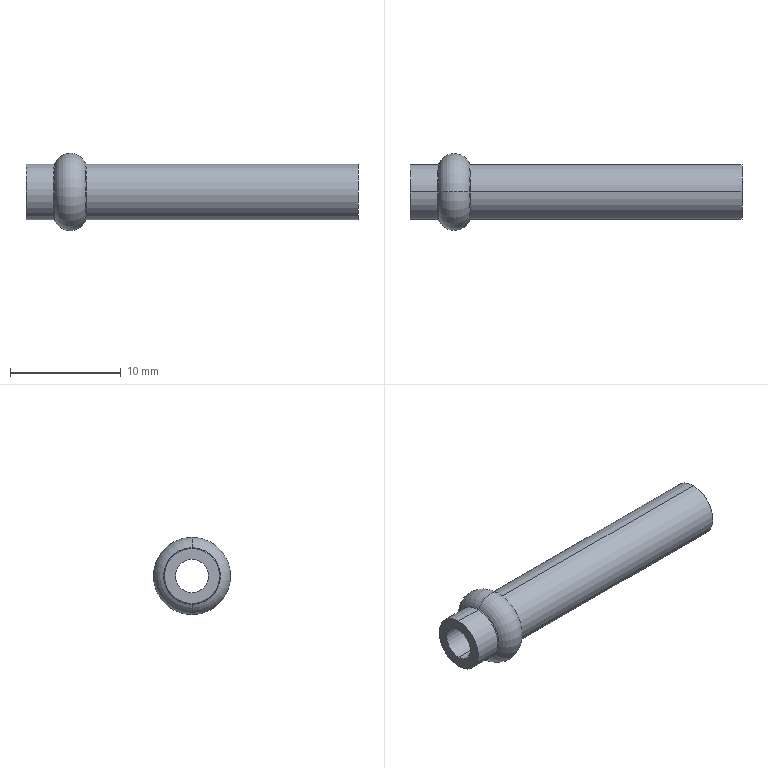Part | SolidWorks | features Fillet 1, Revolution 1 | 1 solid | 14 faces | box 30 x 7 x 7 mm | volume 414.784 mm3 | torus 6 | cylinder 6 | plane 2 | commonest cylinder face diameters 5 x4 3 x2
STEP:
#1=CARTESIAN_POINT('',(2.517,0.,-2.5));
#2=VERTEX_POINT('',#1);
#3=CARTESIAN_POINT('',(2.517,0.,2.5));
#4=VERTEX_POINT('',#3);
#5=CARTESIAN_POINT('',(2.517,0.,0.));
#6=DIRECTION('',(-1.,0.,0.));
#7=DIRECTION('',(0.,0.,1.));
#8=AXIS2_PLACEMENT_3D('',#5,#6,#7);
#9=CIRCLE('',#8,2.5);
#10=EDGE_CURVE('',#2,#4,#9,.T.);
#11=ORIENTED_EDGE('',*,*,#10,.F.);
#12=CARTESIAN_POINT('',(2.609,0.,-2.563));
#13=VERTEX_POINT('',#12);
#14=CARTESIAN_POINT('',(2.517,0.,-2.6));
#15=DIRECTION('',(0.,1.,0.));
#16=DIRECTION('',(0.,0.,1.));
#17=AXIS2_PLACEMENT_3D('',#14,#15,#16);
#18=CIRCLE('',#17,0.1);
#19=EDGE_CURVE('',#2,#13,#18,.T.);
#20=ORIENTED_EDGE('',*,*,#19,.T.);
#21=CARTESIAN_POINT('',(2.609,0.,2.563));
#22=VERTEX_POINT('',#21);
#23=CARTESIAN_POINT('',(2.609,0.,0.));
#24=DIRECTION('',(1.,0.,0.));
#25=DIRECTION('',(0.,0.,-1.));
#26=AXIS2_PLACEMENT_3D('',#23,#24,#25);
#27=CIRCLE('',#26,2.563);
#28=EDGE_CURVE('',#22,#13,#27,.T.);
#29=ORIENTED_EDGE('',*,*,#28,.F.);
#30=CARTESIAN_POINT('',(2.517,0.,2.6));
#31=DIRECTION('',(0.,-1.,0.));
#32=DIRECTION('',(0.,0.,-1.));
#33=AXIS2_PLACEMENT_3D('',#30,#31,#32);
#34=CIRCLE('',#33,0.1);
#35=EDGE_CURVE('',#4,#22,#34,.T.);
#36=ORIENTED_EDGE('',*,*,#35,.F.);
#37=EDGE_LOOP('',(#11,#20,#29,#36));
#38=FACE_OUTER_BOUND('',#37,.T.);
#39=CARTESIAN_POINT('',(2.517,0.,0.));
#40=DIRECTION('',(-1.,0.,0.));
#41=DIRECTION('',(0.,0.,1.));
#42=AXIS2_PLACEMENT_3D('',#39,#40,#41);
#43=TOROIDAL_SURFACE('',#42,2.6,0.1);
#44=ADVANCED_FACE('',(#38),#43,.F.);
#45=CARTESIAN_POINT('',(5.391,0.,-2.563));
#46=VERTEX_POINT('',#45);
#47=CARTESIAN_POINT('',(5.391,0.,2.563));
#48=VERTEX_POINT('',#47);
#49=CARTESIAN_POINT('',(5.391,0.,0.));
#50=DIRECTION('',(-1.,0.,0.));
#51=DIRECTION('',(0.,0.,1.));
#52=AXIS2_PLACEMENT_3D('',#49,#50,#51);
#53=CIRCLE('',#52,2.563);
#54=EDGE_CURVE('',#46,#48,#53,.T.);
#55=ORIENTED_EDGE('',*,*,#54,.F.);
#56=CARTESIAN_POINT('',(5.483,0.,-2.5));
#57=VERTEX_POINT('',#56);
#58=CARTESIAN_POINT('',(5.483,0.,-2.6));
#59=DIRECTION('',(0.,1.,0.));
#60=DIRECTION('',(0.,0.,1.));
#61=AXIS2_PLACEMENT_3D('',#58,#59,#60);
#62=CIRCLE('',#61,0.1);
#63=EDGE_CURVE('',#46,#57,#62,.T.);
#64=ORIENTED_EDGE('',*,*,#63,.T.);
#65=CARTESIAN_POINT('',(5.483,0.,2.5));
#66=VERTEX_POINT('',#65);
#67=CARTESIAN_POINT('',(5.483,0.,0.));
#68=DIRECTION('',(1.,0.,0.));
#69=DIRECTION('',(0.,0.,1.));
#70=AXIS2_PLACEMENT_3D('',#67,#68,#69);
#71=CIRCLE('',#70,2.5);
#72=EDGE_CURVE('',#66,#57,#71,.T.);
#73=ORIENTED_EDGE('',*,*,#72,.F.);
#74=CARTESIAN_POINT('',(5.483,0.,2.6));
#75=DIRECTION('',(0.,-1.,0.));
#76=DIRECTION('',(0.,0.,-1.));
#77=AXIS2_PLACEMENT_3D('',#74,#75,#76);
#78=CIRCLE('',#77,0.1);
#79=EDGE_CURVE('',#48,#66,#78,.T.);
#80=ORIENTED_EDGE('',*,*,#79,.F.);
#81=EDGE_LOOP('',(#55,#64,#73,#80));
#82=FACE_OUTER_BOUND('',#81,.T.);
#83=CARTESIAN_POINT('',(5.483,0.,0.));
#84=DIRECTION('',(-1.,0.,0.));
#85=DIRECTION('',(0.,0.,1.));
#86=AXIS2_PLACEMENT_3D('',#83,#84,#85);
#87=TOROIDAL_SURFACE('',#86,2.6,0.1);
#88=ADVANCED_FACE('',(#82),#87,.F.);
#89=CARTESIAN_POINT('',(2.517,0.,0.));
#90=DIRECTION('',(-1.,0.,0.));
#91=DIRECTION('',(0.,0.,1.));
#92=AXIS2_PLACEMENT_3D('',#89,#90,#91);
#93=CIRCLE('',#92,2.5);
#94=EDGE_CURVE('',#4,#2,#93,.T.);
#95=ORIENTED_EDGE('',*,*,#94,.T.);
#96=CARTESIAN_POINT('',(0.,0.,-2.5));
#97=VERTEX_POINT('',#96);
#98=CARTESIAN_POINT('',(0.,0.,-2.5));
#99=DIRECTION('',(-1.,0.,0.));
#100=VECTOR('',#99,1000.);
#101=LINE('',#98,#100);
#102=EDGE_CURVE('',#2,#97,#101,.T.);
#103=ORIENTED_EDGE('',*,*,#102,.T.);
#104=CARTESIAN_POINT('',(0.,0.,2.5));
#105=VERTEX_POINT('',#104);
#106=CARTESIAN_POINT('',(0.,0.,0.));
#107=DIRECTION('',(-1.,0.,0.));
#108=DIRECTION('',(0.,0.,1.));
#109=AXIS2_PLACEMENT_3D('',#106,#107,#108);
#110=CIRCLE('',#109,2.5);
#111=EDGE_CURVE('',#105,#97,#110,.T.);
#112=ORIENTED_EDGE('',*,*,#111,.F.);
#113=CARTESIAN_POINT('',(0.,0.,2.5));
#114=DIRECTION('',(-1.,0.,0.));
#115=VECTOR('',#114,1000.);
#116=LINE('',#113,#115);
#117=EDGE_CURVE('',#4,#105,#116,.T.);
#118=ORIENTED_EDGE('',*,*,#117,.F.);
#119=EDGE_LOOP('',(#95,#103,#112,#118));
#120=FACE_OUTER_BOUND('',#119,.T.);
#121=CARTESIAN_POINT('',(0.,0.,0.));
#122=DIRECTION('',(-1.,0.,0.));
#123=DIRECTION('',(0.,0.,1.));
#124=AXIS2_PLACEMENT_3D('',#121,#122,#123);
#125=CYLINDRICAL_SURFACE('',#124,2.5);
#126=ADVANCED_FACE('',(#120),#125,.T.);
#127=CARTESIAN_POINT('',(5.391,0.,0.));
#128=DIRECTION('',(-1.,0.,0.));
#129=DIRECTION('',(0.,0.,1.));
#130=AXIS2_PLACEMENT_3D('',#127,#128,#129);
#131=CIRCLE('',#130,2.563);
#132=EDGE_CURVE('',#48,#46,#131,.T.);
#133=ORIENTED_EDGE('',*,*,#132,.T.);
#134=CARTESIAN_POINT('',(4.,0.,-2.));
#135=DIRECTION('',(0.,1.,0.));
#136=DIRECTION('',(0.,0.,1.));
#137=AXIS2_PLACEMENT_3D('',#134,#135,#136);
#138=CIRCLE('',#137,1.5);
#139=EDGE_CURVE('',#46,#13,#138,.T.);
#140=ORIENTED_EDGE('',*,*,#139,.T.);
#141=CARTESIAN_POINT('',(2.609,0.,0.));
#142=DIRECTION('',(1.,0.,0.));
#143=DIRECTION('',(0.,0.,-1.));
#144=AXIS2_PLACEMENT_3D('',#141,#142,#143);
#145=CIRCLE('',#144,2.563);
#146=EDGE_CURVE('',#13,#22,#145,.T.);
#147=ORIENTED_EDGE('',*,*,#146,.T.);
#148=CARTESIAN_POINT('',(4.,0.,2.));
#149=DIRECTION('',(0.,-1.,0.));
#150=DIRECTION('',(0.,0.,-1.));
#151=AXIS2_PLACEMENT_3D('',#148,#149,#150);
#152=CIRCLE('',#151,1.5);
#153=EDGE_CURVE('',#48,#22,#152,.T.);
#154=ORIENTED_EDGE('',*,*,#153,.F.);
#155=EDGE_LOOP('',(#133,#140,#147,#154));
#156=FACE_OUTER_BOUND('',#155,.T.);
#157=CARTESIAN_POINT('',(4.,0.,0.));
#158=DIRECTION('',(-1.,0.,0.));
#159=DIRECTION('',(0.,0.,1.));
#160=AXIS2_PLACEMENT_3D('',#157,#158,#159);
#161=TOROIDAL_SURFACE('',#160,2.,1.5);
#162=ADVANCED_FACE('',(#156),#161,.T.);
#163=CARTESIAN_POINT('',(30.,0.,2.5));
#164=VERTEX_POINT('',#163);
#165=CARTESIAN_POINT('',(30.,0.,-2.5));
#166=VERTEX_POINT('',#165);
#167=CARTESIAN_POINT('',(30.,0.,0.));
#168=DIRECTION('',(-1.,0.,0.));
#169=DIRECTION('',(0.,0.,1.));
#170=AXIS2_PLACEMENT_3D('',#167,#168,#169);
#171=CIRCLE('',#170,2.5);
#172=EDGE_CURVE('',#164,#166,#171,.T.);
#173=ORIENTED_EDGE('',*,*,#172,.T.);
#174=CARTESIAN_POINT('',(0.,0.,-2.5));
#175=DIRECTION('',(-1.,0.,0.));
#176=VECTOR('',#175,1000.);
#177=LINE('',#174,#176);
#178=EDGE_CURVE('',#166,#57,#177,.T.);
#179=ORIENTED_EDGE('',*,*,#178,.T.);
#180=CARTESIAN_POINT('',(5.483,0.,0.));
#181=DIRECTION('',(1.,0.,0.));
#182=DIRECTION('',(0.,0.,1.));
#183=AXIS2_PLACEMENT_3D('',#180,#181,#182);
#184=CIRCLE('',#183,2.5);
#185=EDGE_CURVE('',#57,#66,#184,.T.);
#186=ORIENTED_EDGE('',*,*,#185,.T.);
#187=CARTESIAN_POINT('',(0.,0.,2.5));
#188=DIRECTION('',(-1.,0.,0.));
#189=VECTOR('',#188,1000.);
#190=LINE('',#187,#189);
#191=EDGE_CURVE('',#164,#66,#190,.T.);
#192=ORIENTED_EDGE('',*,*,#191,.F.);
#193=EDGE_LOOP('',(#173,#179,#186,#192));
#194=FACE_OUTER_BOUND('',#193,.T.);
#195=CARTESIAN_POINT('',(0.,0.,0.));
#196=DIRECTION('',(-1.,0.,0.));
#197=DIRECTION('',(0.,0.,1.));
#198=AXIS2_PLACEMENT_3D('',#195,#196,#197);
#199=CYLINDRICAL_SURFACE('',#198,2.5);
#200=ADVANCED_FACE('',(#194),#199,.T.);
#201=CARTESIAN_POINT('',(30.,0.,-1.5));
#202=VERTEX_POINT('',#201);
#203=CARTESIAN_POINT('',(30.,0.,1.5));
#204=VERTEX_POINT('',#203);
#205=CARTESIAN_POINT('',(30.,0.,0.));
#206=DIRECTION('',(-1.,0.,0.));
#207=DIRECTION('',(0.,0.,1.));
#208=AXIS2_PLACEMENT_3D('',#205,#206,#207);
#209=CIRCLE('',#208,1.5);
#210=EDGE_CURVE('',#202,#204,#209,.T.);
#211=ORIENTED_EDGE('',*,*,#210,.F.);
#212=CARTESIAN_POINT('',(0.,0.,-1.5));
#213=VERTEX_POINT('',#212);
#214=CARTESIAN_POINT('',(0.,0.,-1.5));
#215=DIRECTION('',(-1.,0.,0.));
#216=VECTOR('',#215,1000.);
#217=LINE('',#214,#216);
#218=EDGE_CURVE('',#202,#213,#217,.T.);
#219=ORIENTED_EDGE('',*,*,#218,.T.);
#220=CARTESIAN_POINT('',(0.,0.,1.5));
#221=VERTEX_POINT('',#220);
#222=CARTESIAN_POINT('',(0.,0.,0.));
#223=DIRECTION('',(-1.,0.,0.));
#224=DIRECTION('',(0.,0.,1.));
#225=AXIS2_PLACEMENT_3D('',#222,#223,#224);
#226=CIRCLE('',#225,1.5);
#227=EDGE_CURVE('',#213,#221,#226,.T.);
#228=ORIENTED_EDGE('',*,*,#227,.T.);
#229=CARTESIAN_POINT('',(0.,0.,1.5));
#230=DIRECTION('',(-1.,0.,0.));
#231=VECTOR('',#230,1000.);
#232=LINE('',#229,#231);
#233=EDGE_CURVE('',#204,#221,#232,.T.);
#234=ORIENTED_EDGE('',*,*,#233,.F.);
#235=EDGE_LOOP('',(#211,#219,#228,#234));
#236=FACE_OUTER_BOUND('',#235,.T.);
#237=CARTESIAN_POINT('',(0.,0.,0.));
#238=DIRECTION('',(-1.,0.,0.));
#239=DIRECTION('',(0.,0.,1.));
#240=AXIS2_PLACEMENT_3D('',#237,#238,#239);
#241=CYLINDRICAL_SURFACE('',#240,1.5);
#242=ADVANCED_FACE('',(#236),#241,.F.);
#243=CARTESIAN_POINT('',(0.,0.,0.));
#244=DIRECTION('',(-1.,0.,0.));
#245=DIRECTION('',(0.,0.,1.));
#246=AXIS2_PLACEMENT_3D('',#243,#244,#245);
#247=CIRCLE('',#246,1.5);
#248=EDGE_CURVE('',#221,#213,#247,.T.);
#249=ORIENTED_EDGE('',*,*,#248,.F.);
#250=ORIENTED_EDGE('',*,*,#227,.F.);
#251=EDGE_LOOP('',(#249,#250));
#252=FACE_BOUND('',#251,.T.);
#253=ORIENTED_EDGE('',*,*,#111,.T.);
#254=CARTESIAN_POINT('',(0.,0.,0.));
#255=DIRECTION('',(-1.,0.,0.));
#256=DIRECTION('',(0.,0.,1.));
#257=AXIS2_PLACEMENT_3D('',#254,#255,#256);
#258=CIRCLE('',#257,2.5);
#259=EDGE_CURVE('',#97,#105,#258,.T.);
#260=ORIENTED_EDGE('',*,*,#259,.T.);
#261=EDGE_LOOP('',(#253,#260));
#262=FACE_OUTER_BOUND('',#261,.T.);
#263=CARTESIAN_POINT('',(0.,1.5,0.));
#264=DIRECTION('',(1.,0.,0.));
#265=DIRECTION('',(0.,0.,-1.));
#266=AXIS2_PLACEMENT_3D('',#263,#264,#265);
#267=PLANE('',#266);
#268=ADVANCED_FACE('',(#252,#262),#267,.F.);
#269=ORIENTED_EDGE('',*,*,#218,.F.);
#270=CARTESIAN_POINT('',(30.,0.,0.));
#271=DIRECTION('',(-1.,0.,0.));
#272=DIRECTION('',(0.,0.,1.));
#273=AXIS2_PLACEMENT_3D('',#270,#271,#272);
#274=CIRCLE('',#273,1.5);
#275=EDGE_CURVE('',#204,#202,#274,.T.);
#276=ORIENTED_EDGE('',*,*,#275,.F.);
#277=ORIENTED_EDGE('',*,*,#233,.T.);
#278=ORIENTED_EDGE('',*,*,#248,.T.);
#279=EDGE_LOOP('',(#269,#276,#277,#278));
#280=FACE_OUTER_BOUND('',#279,.T.);
#281=CARTESIAN_POINT('',(0.,0.,0.));
#282=DIRECTION('',(-1.,0.,0.));
#283=DIRECTION('',(0.,0.,1.));
#284=AXIS2_PLACEMENT_3D('',#281,#282,#283);
#285=CYLINDRICAL_SURFACE('',#284,1.5);
#286=ADVANCED_FACE('',(#280),#285,.F.);
#287=ORIENTED_EDGE('',*,*,#172,.F.);
#288=CARTESIAN_POINT('',(30.,0.,0.));
#289=DIRECTION('',(-1.,0.,0.));
#290=DIRECTION('',(0.,0.,1.));
#291=AXIS2_PLACEMENT_3D('',#288,#289,#290);
#292=CIRCLE('',#291,2.5);
#293=EDGE_CURVE('',#166,#164,#292,.T.);
#294=ORIENTED_EDGE('',*,*,#293,.F.);
#295=EDGE_LOOP('',(#287,#294));
#296=FACE_OUTER_BOUND('',#295,.T.);
#297=ORIENTED_EDGE('',*,*,#275,.T.);
#298=ORIENTED_EDGE('',*,*,#210,.T.);
#299=EDGE_LOOP('',(#297,#298));
#300=FACE_BOUND('',#299,.T.);
#301=CARTESIAN_POINT('',(30.,2.5,0.));
#302=DIRECTION('',(-1.,0.,0.));
#303=DIRECTION('',(0.,0.,1.));
#304=AXIS2_PLACEMENT_3D('',#301,#302,#303);
#305=PLANE('',#304);
#306=ADVANCED_FACE('',(#296,#300),#305,.F.);
#307=ORIENTED_EDGE('',*,*,#178,.F.);
#308=ORIENTED_EDGE('',*,*,#293,.T.);
#309=ORIENTED_EDGE('',*,*,#191,.T.);
#310=ORIENTED_EDGE('',*,*,#72,.T.);
#311=EDGE_LOOP('',(#307,#308,#309,#310));
#312=FACE_OUTER_BOUND('',#311,.T.);
#313=CARTESIAN_POINT('',(0.,0.,0.));
#314=DIRECTION('',(-1.,0.,0.));
#315=DIRECTION('',(0.,0.,1.));
#316=AXIS2_PLACEMENT_3D('',#313,#314,#315);
#317=CYLINDRICAL_SURFACE('',#316,2.5);
#318=ADVANCED_FACE('',(#312),#317,.T.);
#319=ORIENTED_EDGE('',*,*,#139,.F.);
#320=ORIENTED_EDGE('',*,*,#54,.T.);
#321=ORIENTED_EDGE('',*,*,#153,.T.);
#322=ORIENTED_EDGE('',*,*,#28,.T.);
#323=EDGE_LOOP('',(#319,#320,#321,#322));
#324=FACE_OUTER_BOUND('',#323,.T.);
#325=CARTESIAN_POINT('',(4.,0.,0.));
#326=DIRECTION('',(-1.,0.,0.));
#327=DIRECTION('',(0.,0.,1.));
#328=AXIS2_PLACEMENT_3D('',#325,#326,#327);
#329=TOROIDAL_SURFACE('',#328,2.,1.5);
#330=ADVANCED_FACE('',(#324),#329,.T.);
#331=ORIENTED_EDGE('',*,*,#102,.F.);
#332=ORIENTED_EDGE('',*,*,#10,.T.);
#333=ORIENTED_EDGE('',*,*,#117,.T.);
#334=ORIENTED_EDGE('',*,*,#259,.F.);
#335=EDGE_LOOP('',(#331,#332,#333,#334));
#336=FACE_OUTER_BOUND('',#335,.T.);
#337=CARTESIAN_POINT('',(0.,0.,0.));
#338=DIRECTION('',(-1.,0.,0.));
#339=DIRECTION('',(0.,0.,1.));
#340=AXIS2_PLACEMENT_3D('',#337,#338,#339);
#341=CYLINDRICAL_SURFACE('',#340,2.5);
#342=ADVANCED_FACE('',(#336),#341,.T.);
#343=ORIENTED_EDGE('',*,*,#63,.F.);
#344=ORIENTED_EDGE('',*,*,#132,.F.);
#345=ORIENTED_EDGE('',*,*,#79,.T.);
#346=ORIENTED_EDGE('',*,*,#185,.F.);
#347=EDGE_LOOP('',(#343,#344,#345,#346));
#348=FACE_OUTER_BOUND('',#347,.T.);
#349=CARTESIAN_POINT('',(5.483,0.,0.));
#350=DIRECTION('',(-1.,0.,0.));
#351=DIRECTION('',(0.,0.,1.));
#352=AXIS2_PLACEMENT_3D('',#349,#350,#351);
#353=TOROIDAL_SURFACE('',#352,2.6,0.1);
#354=ADVANCED_FACE('',(#348),#353,.F.);
#355=ORIENTED_EDGE('',*,*,#19,.F.);
#356=ORIENTED_EDGE('',*,*,#94,.F.);
#357=ORIENTED_EDGE('',*,*,#35,.T.);
#358=ORIENTED_EDGE('',*,*,#146,.F.);
#359=EDGE_LOOP('',(#355,#356,#357,#358));
#360=FACE_OUTER_BOUND('',#359,.T.);
#361=CARTESIAN_POINT('',(2.517,0.,0.));
#362=DIRECTION('',(-1.,0.,0.));
#363=DIRECTION('',(0.,0.,1.));
#364=AXIS2_PLACEMENT_3D('',#361,#362,#363);
#365=TOROIDAL_SURFACE('',#364,2.6,0.1);
#366=ADVANCED_FACE('',(#360),#365,.F.);
#367=CLOSED_SHELL('',(#44,#88,#126,#162,#200,#242,#268,#286,#306,#318,#330,#342,#354,#366));
#368=MANIFOLD_SOLID_BREP('',#367);
#369=CARTESIAN_POINT('',(0.,0.,0.));
#370=DIRECTION('',(0.,0.,1.));
#371=DIRECTION('',(1.,0.,0.));
#372=AXIS2_PLACEMENT_3D('',#369,#370,#371);
#373=(LENGTH_UNIT()NAMED_UNIT(*)SI_UNIT(.MILLI.,.METRE.));
#374=UNCERTAINTY_MEASURE_WITH_UNIT(LENGTH_MEASURE(0.00001),#373,'','');
#375=(NAMED_UNIT(*)PLANE_ANGLE_UNIT()SI_UNIT($,.RADIAN.));
#376=(NAMED_UNIT(*)SI_UNIT($,.STERADIAN.)SOLID_ANGLE_UNIT());
#377=(GEOMETRIC_REPRESENTATION_CONTEXT(3)GLOBAL_UNCERTAINTY_ASSIGNED_CONTEXT((#374))GLOBAL_UNIT_ASSIGNED_CONTEXT((#373,#375,#376))REPRESENTATION_CONTEXT('',''));
#378=ADVANCED_BREP_SHAPE_REPRESENTATION('',(#368,#372),#377);